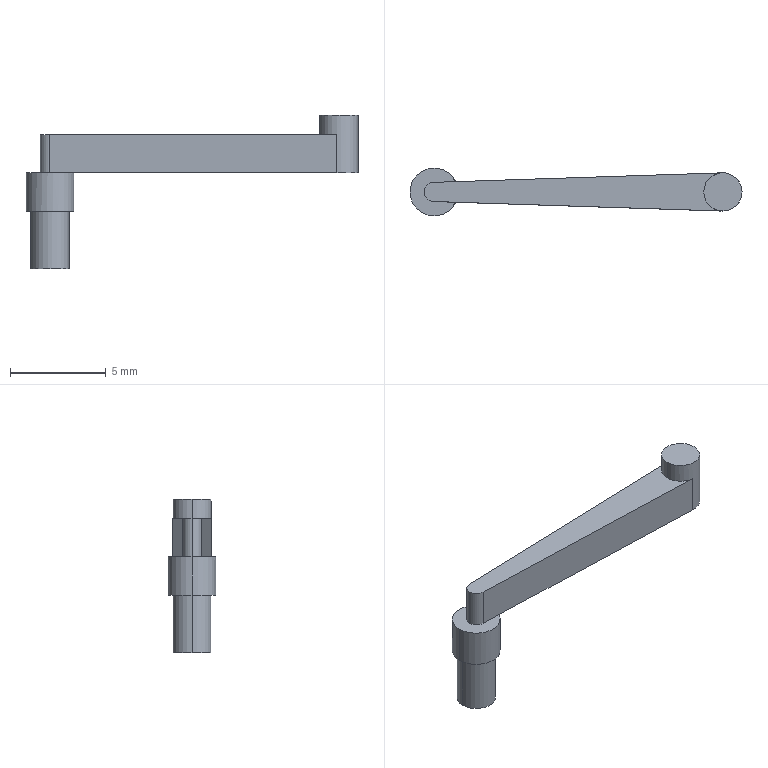Part | SolidWorks | features ICE 5, Extrusion 1 | 1 solid | 16 faces | box 17.35 x 2.5 x 8 mm | volume 71.56 mm3 | cylinder 8 | plane 8 | commonest cylinder face diameters 2 x4 1 x2 2.5 x2
STEP:
#1=CARTESIAN_POINT('',(-1.,0.,-4.));
#2=VERTEX_POINT('',#1);
#3=CARTESIAN_POINT('',(1.,0.,-4.));
#4=VERTEX_POINT('',#3);
#5=CARTESIAN_POINT('',(0.,0.,-4.));
#6=DIRECTION('',(0.,0.,-1.));
#7=DIRECTION('',(-1.,0.,0.));
#8=AXIS2_PLACEMENT_3D('',#5,#6,#7);
#9=CIRCLE('',#8,1.);
#10=EDGE_CURVE('',#2,#4,#9,.T.);
#11=ORIENTED_EDGE('',*,*,#10,.F.);
#12=CARTESIAN_POINT('',(-1.,0.,-1.));
#13=VERTEX_POINT('',#12);
#14=CARTESIAN_POINT('',(-1.,0.,-4.));
#15=DIRECTION('',(0.,0.,1.));
#16=VECTOR('',#15,1000.);
#17=LINE('',#14,#16);
#18=EDGE_CURVE('',#2,#13,#17,.T.);
#19=ORIENTED_EDGE('',*,*,#18,.T.);
#20=CARTESIAN_POINT('',(1.,0.,-1.));
#21=VERTEX_POINT('',#20);
#22=CARTESIAN_POINT('',(0.,0.,-1.));
#23=DIRECTION('',(0.,0.,-1.));
#24=DIRECTION('',(-1.,0.,0.));
#25=AXIS2_PLACEMENT_3D('',#22,#23,#24);
#26=CIRCLE('',#25,1.);
#27=EDGE_CURVE('',#13,#21,#26,.T.);
#28=ORIENTED_EDGE('',*,*,#27,.T.);
#29=CARTESIAN_POINT('',(1.,0.,-4.));
#30=DIRECTION('',(0.,0.,1.));
#31=VECTOR('',#30,1000.);
#32=LINE('',#29,#31);
#33=EDGE_CURVE('',#4,#21,#32,.T.);
#34=ORIENTED_EDGE('',*,*,#33,.F.);
#35=EDGE_LOOP('',(#11,#19,#28,#34));
#36=FACE_OUTER_BOUND('',#35,.T.);
#37=CARTESIAN_POINT('',(0.,0.,-4.));
#38=DIRECTION('',(0.,0.,1.));
#39=DIRECTION('',(1.,0.,0.));
#40=AXIS2_PLACEMENT_3D('',#37,#38,#39);
#41=CYLINDRICAL_SURFACE('',#40,1.);
#42=ADVANCED_FACE('',(#36),#41,.T.);
#43=CARTESIAN_POINT('',(1.25,0.,-1.));
#44=VERTEX_POINT('',#43);
#45=CARTESIAN_POINT('',(-1.25,0.,-1.));
#46=VERTEX_POINT('',#45);
#47=CARTESIAN_POINT('',(0.,0.,-1.));
#48=DIRECTION('',(0.,0.,1.));
#49=DIRECTION('',(1.,0.,0.));
#50=AXIS2_PLACEMENT_3D('',#47,#48,#49);
#51=CIRCLE('',#50,1.25);
#52=EDGE_CURVE('',#44,#46,#51,.T.);
#53=ORIENTED_EDGE('',*,*,#52,.T.);
#54=CARTESIAN_POINT('',(-1.25,0.,1.));
#55=VERTEX_POINT('',#54);
#56=CARTESIAN_POINT('',(-1.25,0.,-1.));
#57=DIRECTION('',(0.,0.,1.));
#58=VECTOR('',#57,1000.);
#59=LINE('',#56,#58);
#60=EDGE_CURVE('',#46,#55,#59,.T.);
#61=ORIENTED_EDGE('',*,*,#60,.T.);
#62=CARTESIAN_POINT('',(1.129,0.5372,1.));
#63=VERTEX_POINT('',#62);
#64=CARTESIAN_POINT('',(0.,0.,1.));
#65=DIRECTION('',(0.,0.,1.));
#66=DIRECTION('',(1.,0.,0.));
#67=AXIS2_PLACEMENT_3D('',#64,#65,#66);
#68=CIRCLE('',#67,1.25);
#69=EDGE_CURVE('',#63,#55,#68,.T.);
#70=ORIENTED_EDGE('',*,*,#69,.F.);
#71=CARTESIAN_POINT('',(1.25,0.,1.));
#72=VERTEX_POINT('',#71);
#73=CARTESIAN_POINT('',(0.,0.,1.));
#74=DIRECTION('',(0.,0.,1.));
#75=DIRECTION('',(1.,0.,0.));
#76=AXIS2_PLACEMENT_3D('',#73,#74,#75);
#77=CIRCLE('',#76,1.25);
#78=EDGE_CURVE('',#72,#63,#77,.T.);
#79=ORIENTED_EDGE('',*,*,#78,.F.);
#80=CARTESIAN_POINT('',(1.25,0.,-1.));
#81=DIRECTION('',(0.,0.,1.));
#82=VECTOR('',#81,1000.);
#83=LINE('',#80,#82);
#84=EDGE_CURVE('',#44,#72,#83,.T.);
#85=ORIENTED_EDGE('',*,*,#84,.F.);
#86=EDGE_LOOP('',(#53,#61,#70,#79,#85));
#87=FACE_OUTER_BOUND('',#86,.T.);
#88=CARTESIAN_POINT('',(0.,0.,-1.));
#89=DIRECTION('',(0.,0.,1.));
#90=DIRECTION('',(1.,0.,0.));
#91=AXIS2_PLACEMENT_3D('',#88,#89,#90);
#92=CYLINDRICAL_SURFACE('',#91,1.25);
#93=ADVANCED_FACE('',(#87),#92,.T.);
#94=CARTESIAN_POINT('',(16.1,0.,4.));
#95=VERTEX_POINT('',#94);
#96=CARTESIAN_POINT('',(14.1,0.,4.));
#97=VERTEX_POINT('',#96);
#98=CARTESIAN_POINT('',(15.1,0.,4.));
#99=DIRECTION('',(0.,0.,1.));
#100=DIRECTION('',(1.,0.,0.));
#101=AXIS2_PLACEMENT_3D('',#98,#99,#100);
#102=CIRCLE('',#101,1.);
#103=EDGE_CURVE('',#95,#97,#102,.T.);
#104=ORIENTED_EDGE('',*,*,#103,.F.);
#105=CARTESIAN_POINT('',(16.1,0.,1.));
#106=VERTEX_POINT('',#105);
#107=CARTESIAN_POINT('',(16.1,0.,3.));
#108=DIRECTION('',(0.,0.,-1.));
#109=VECTOR('',#108,1000.);
#110=LINE('',#107,#109);
#111=EDGE_CURVE('',#95,#106,#110,.T.);
#112=ORIENTED_EDGE('',*,*,#111,.T.);
#113=CARTESIAN_POINT('',(15.,0.995,1.));
#114=VERTEX_POINT('',#113);
#115=CARTESIAN_POINT('',(15.1,0.,1.));
#116=DIRECTION('',(0.,0.,1.));
#117=DIRECTION('',(1.,0.,0.));
#118=AXIS2_PLACEMENT_3D('',#115,#116,#117);
#119=CIRCLE('',#118,1.);
#120=EDGE_CURVE('',#106,#114,#119,.T.);
#121=ORIENTED_EDGE('',*,*,#120,.T.);
#122=CARTESIAN_POINT('',(15.,0.995,3.));
#123=VERTEX_POINT('',#122);
#124=CARTESIAN_POINT('',(15.,0.995,3.));
#125=DIRECTION('',(0.,0.,-1.));
#126=VECTOR('',#125,1000.);
#127=LINE('',#124,#126);
#128=EDGE_CURVE('',#123,#114,#127,.T.);
#129=ORIENTED_EDGE('',*,*,#128,.F.);
#130=CARTESIAN_POINT('',(14.1,0.,3.));
#131=VERTEX_POINT('',#130);
#132=CARTESIAN_POINT('',(15.1,0.,3.));
#133=DIRECTION('',(0.,0.,1.));
#134=DIRECTION('',(1.,0.,0.));
#135=AXIS2_PLACEMENT_3D('',#132,#133,#134);
#136=CIRCLE('',#135,1.);
#137=EDGE_CURVE('',#123,#131,#136,.T.);
#138=ORIENTED_EDGE('',*,*,#137,.T.);
#139=CARTESIAN_POINT('',(14.1,0.,3.));
#140=DIRECTION('',(0.,0.,-1.));
#141=VECTOR('',#140,1000.);
#142=LINE('',#139,#141);
#143=EDGE_CURVE('',#97,#131,#142,.T.);
#144=ORIENTED_EDGE('',*,*,#143,.F.);
#145=EDGE_LOOP('',(#104,#112,#121,#129,#138,#144));
#146=FACE_OUTER_BOUND('',#145,.T.);
#147=CARTESIAN_POINT('',(15.1,0.,3.));
#148=DIRECTION('',(0.,0.,-1.));
#149=DIRECTION('',(-1.,0.,0.));
#150=AXIS2_PLACEMENT_3D('',#147,#148,#149);
#151=CYLINDRICAL_SURFACE('',#150,1.);
#152=ADVANCED_FACE('',(#146),#151,.T.);
#153=CARTESIAN_POINT('',(-0.5,0.,3.));
#154=VERTEX_POINT('',#153);
#155=CARTESIAN_POINT('',(0.,-0.5,3.));
#156=VERTEX_POINT('',#155);
#157=CARTESIAN_POINT('',(0.,0.,3.));
#158=DIRECTION('',(0.,0.,1.));
#159=DIRECTION('',(1.,0.,0.));
#160=AXIS2_PLACEMENT_3D('',#157,#158,#159);
#161=CIRCLE('',#160,0.5);
#162=EDGE_CURVE('',#154,#156,#161,.T.);
#163=ORIENTED_EDGE('',*,*,#162,.F.);
#164=CARTESIAN_POINT('',(-0.5,0.,1.));
#165=VERTEX_POINT('',#164);
#166=CARTESIAN_POINT('',(-0.5,0.,3.));
#167=DIRECTION('',(0.,0.,-1.));
#168=VECTOR('',#167,1000.);
#169=LINE('',#166,#168);
#170=EDGE_CURVE('',#154,#165,#169,.T.);
#171=ORIENTED_EDGE('',*,*,#170,.T.);
#172=CARTESIAN_POINT('',(0.,-0.5,1.));
#173=VERTEX_POINT('',#172);
#174=CARTESIAN_POINT('',(0.,0.,1.));
#175=DIRECTION('',(0.,0.,1.));
#176=DIRECTION('',(1.,0.,0.));
#177=AXIS2_PLACEMENT_3D('',#174,#175,#176);
#178=CIRCLE('',#177,0.5);
#179=EDGE_CURVE('',#165,#173,#178,.T.);
#180=ORIENTED_EDGE('',*,*,#179,.T.);
#181=CARTESIAN_POINT('',(0.,-0.5,3.));
#182=DIRECTION('',(0.,0.,-1.));
#183=VECTOR('',#182,1000.);
#184=LINE('',#181,#183);
#185=EDGE_CURVE('',#156,#173,#184,.T.);
#186=ORIENTED_EDGE('',*,*,#185,.F.);
#187=EDGE_LOOP('',(#163,#171,#180,#186));
#188=FACE_OUTER_BOUND('',#187,.T.);
#189=CARTESIAN_POINT('',(0.,0.,3.));
#190=DIRECTION('',(0.,0.,-1.));
#191=DIRECTION('',(-1.,0.,0.));
#192=AXIS2_PLACEMENT_3D('',#189,#190,#191);
#193=CYLINDRICAL_SURFACE('',#192,0.5);
#194=ADVANCED_FACE('',(#188),#193,.T.);
#195=CARTESIAN_POINT('',(0.,0.5,1.));
#196=VERTEX_POINT('',#195);
#197=CARTESIAN_POINT('',(0.,0.5,1.));
#198=DIRECTION('',(-0.9995,-0.03298,0.));
#199=VECTOR('',#198,1000.);
#200=LINE('',#197,#199);
#201=EDGE_CURVE('',#63,#196,#200,.T.);
#202=ORIENTED_EDGE('',*,*,#201,.F.);
#203=ORIENTED_EDGE('',*,*,#69,.T.);
#204=CARTESIAN_POINT('',(1.129,-0.5372,1.));
#205=VERTEX_POINT('',#204);
#206=CARTESIAN_POINT('',(0.,0.,1.));
#207=DIRECTION('',(0.,0.,1.));
#208=DIRECTION('',(1.,0.,0.));
#209=AXIS2_PLACEMENT_3D('',#206,#207,#208);
#210=CIRCLE('',#209,1.25);
#211=EDGE_CURVE('',#55,#205,#210,.T.);
#212=ORIENTED_EDGE('',*,*,#211,.T.);
#213=CARTESIAN_POINT('',(0.,-0.5,1.));
#214=DIRECTION('',(0.9995,-0.03298,0.));
#215=VECTOR('',#214,1000.);
#216=LINE('',#213,#215);
#217=EDGE_CURVE('',#173,#205,#216,.T.);
#218=ORIENTED_EDGE('',*,*,#217,.F.);
#219=ORIENTED_EDGE('',*,*,#179,.F.);
#220=CARTESIAN_POINT('',(0.,0.,1.));
#221=DIRECTION('',(0.,0.,1.));
#222=DIRECTION('',(1.,0.,0.));
#223=AXIS2_PLACEMENT_3D('',#220,#221,#222);
#224=CIRCLE('',#223,0.5);
#225=EDGE_CURVE('',#196,#165,#224,.T.);
#226=ORIENTED_EDGE('',*,*,#225,.F.);
#227=EDGE_LOOP('',(#202,#203,#212,#218,#219,#226));
#228=FACE_OUTER_BOUND('',#227,.T.);
#229=CARTESIAN_POINT('',(0.,0.,1.));
#230=DIRECTION('',(0.,0.,1.));
#231=DIRECTION('',(1.,0.,0.));
#232=AXIS2_PLACEMENT_3D('',#229,#230,#231);
#233=PLANE('',#232);
#234=ADVANCED_FACE('',(#228),#233,.T.);
#235=CARTESIAN_POINT('',(0.,0.,1.));
#236=DIRECTION('',(0.,0.,1.));
#237=DIRECTION('',(1.,0.,0.));
#238=AXIS2_PLACEMENT_3D('',#235,#236,#237);
#239=CIRCLE('',#238,1.25);
#240=EDGE_CURVE('',#205,#72,#239,.T.);
#241=ORIENTED_EDGE('',*,*,#240,.T.);
#242=ORIENTED_EDGE('',*,*,#78,.T.);
#243=CARTESIAN_POINT('',(0.,0.5,1.));
#244=DIRECTION('',(-0.9995,-0.03298,0.));
#245=VECTOR('',#244,1000.);
#246=LINE('',#243,#245);
#247=EDGE_CURVE('',#114,#63,#246,.T.);
#248=ORIENTED_EDGE('',*,*,#247,.F.);
#249=ORIENTED_EDGE('',*,*,#120,.F.);
#250=CARTESIAN_POINT('',(15.,-0.995,1.));
#251=VERTEX_POINT('',#250);
#252=CARTESIAN_POINT('',(15.1,0.,1.));
#253=DIRECTION('',(0.,0.,1.));
#254=DIRECTION('',(1.,0.,0.));
#255=AXIS2_PLACEMENT_3D('',#252,#253,#254);
#256=CIRCLE('',#255,1.);
#257=EDGE_CURVE('',#251,#106,#256,.T.);
#258=ORIENTED_EDGE('',*,*,#257,.F.);
#259=CARTESIAN_POINT('',(0.,-0.5,1.));
#260=DIRECTION('',(0.9995,-0.03298,0.));
#261=VECTOR('',#260,1000.);
#262=LINE('',#259,#261);
#263=EDGE_CURVE('',#205,#251,#262,.T.);
#264=ORIENTED_EDGE('',*,*,#263,.F.);
#265=EDGE_LOOP('',(#241,#242,#248,#249,#258,#264));
#266=FACE_OUTER_BOUND('',#265,.T.);
#267=CARTESIAN_POINT('',(0.,0.,1.));
#268=DIRECTION('',(0.,0.,1.));
#269=DIRECTION('',(1.,0.,0.));
#270=AXIS2_PLACEMENT_3D('',#267,#268,#269);
#271=PLANE('',#270);
#272=ADVANCED_FACE('',(#266),#271,.F.);
#273=ORIENTED_EDGE('',*,*,#170,.F.);
#274=CARTESIAN_POINT('',(0.,0.5,3.));
#275=VERTEX_POINT('',#274);
#276=CARTESIAN_POINT('',(0.,0.,3.));
#277=DIRECTION('',(0.,0.,1.));
#278=DIRECTION('',(1.,0.,0.));
#279=AXIS2_PLACEMENT_3D('',#276,#277,#278);
#280=CIRCLE('',#279,0.5);
#281=EDGE_CURVE('',#275,#154,#280,.T.);
#282=ORIENTED_EDGE('',*,*,#281,.F.);
#283=CARTESIAN_POINT('',(0.,0.5,3.));
#284=DIRECTION('',(0.,0.,-1.));
#285=VECTOR('',#284,1000.);
#286=LINE('',#283,#285);
#287=EDGE_CURVE('',#275,#196,#286,.T.);
#288=ORIENTED_EDGE('',*,*,#287,.T.);
#289=ORIENTED_EDGE('',*,*,#225,.T.);
#290=EDGE_LOOP('',(#273,#282,#288,#289));
#291=FACE_OUTER_BOUND('',#290,.T.);
#292=CARTESIAN_POINT('',(0.,0.,3.));
#293=DIRECTION('',(0.,0.,-1.));
#294=DIRECTION('',(-1.,0.,0.));
#295=AXIS2_PLACEMENT_3D('',#292,#293,#294);
#296=CYLINDRICAL_SURFACE('',#295,0.5);
#297=ADVANCED_FACE('',(#291),#296,.T.);
#298=ORIENTED_EDGE('',*,*,#217,.T.);
#299=ORIENTED_EDGE('',*,*,#263,.T.);
#300=CARTESIAN_POINT('',(15.,-0.995,3.));
#301=VERTEX_POINT('',#300);
#302=CARTESIAN_POINT('',(15.,-0.995,3.));
#303=DIRECTION('',(0.,0.,-1.));
#304=VECTOR('',#303,1000.);
#305=LINE('',#302,#304);
#306=EDGE_CURVE('',#301,#251,#305,.T.);
#307=ORIENTED_EDGE('',*,*,#306,.F.);
#308=CARTESIAN_POINT('',(0.,-0.5,3.));
#309=DIRECTION('',(0.9995,-0.03298,0.));
#310=VECTOR('',#309,1000.);
#311=LINE('',#308,#310);
#312=EDGE_CURVE('',#156,#301,#311,.T.);
#313=ORIENTED_EDGE('',*,*,#312,.F.);
#314=ORIENTED_EDGE('',*,*,#185,.T.);
#315=EDGE_LOOP('',(#298,#299,#307,#313,#314));
#316=FACE_OUTER_BOUND('',#315,.T.);
#317=CARTESIAN_POINT('',(0.,-0.5,3.));
#318=DIRECTION('',(0.03298,0.9995,0.));
#319=DIRECTION('',(-0.9995,0.03298,0.));
#320=AXIS2_PLACEMENT_3D('',#317,#318,#319);
#321=PLANE('',#320);
#322=ADVANCED_FACE('',(#316),#321,.F.);
#323=ORIENTED_EDGE('',*,*,#111,.F.);
#324=CARTESIAN_POINT('',(15.1,0.,4.));
#325=DIRECTION('',(0.,0.,1.));
#326=DIRECTION('',(1.,0.,0.));
#327=AXIS2_PLACEMENT_3D('',#324,#325,#326);
#328=CIRCLE('',#327,1.);
#329=EDGE_CURVE('',#97,#95,#328,.T.);
#330=ORIENTED_EDGE('',*,*,#329,.F.);
#331=ORIENTED_EDGE('',*,*,#143,.T.);
#332=CARTESIAN_POINT('',(15.1,0.,3.));
#333=DIRECTION('',(0.,0.,1.));
#334=DIRECTION('',(1.,0.,0.));
#335=AXIS2_PLACEMENT_3D('',#332,#333,#334);
#336=CIRCLE('',#335,1.);
#337=EDGE_CURVE('',#131,#301,#336,.T.);
#338=ORIENTED_EDGE('',*,*,#337,.T.);
#339=ORIENTED_EDGE('',*,*,#306,.T.);
#340=ORIENTED_EDGE('',*,*,#257,.T.);
#341=EDGE_LOOP('',(#323,#330,#331,#338,#339,#340));
#342=FACE_OUTER_BOUND('',#341,.T.);
#343=CARTESIAN_POINT('',(15.1,0.,3.));
#344=DIRECTION('',(0.,0.,-1.));
#345=DIRECTION('',(-1.,0.,0.));
#346=AXIS2_PLACEMENT_3D('',#343,#344,#345);
#347=CYLINDRICAL_SURFACE('',#346,1.);
#348=ADVANCED_FACE('',(#342),#347,.T.);
#349=ORIENTED_EDGE('',*,*,#247,.T.);
#350=ORIENTED_EDGE('',*,*,#201,.T.);
#351=ORIENTED_EDGE('',*,*,#287,.F.);
#352=CARTESIAN_POINT('',(0.,0.5,3.));
#353=DIRECTION('',(-0.9995,-0.03298,0.));
#354=VECTOR('',#353,1000.);
#355=LINE('',#352,#354);
#356=EDGE_CURVE('',#123,#275,#355,.T.);
#357=ORIENTED_EDGE('',*,*,#356,.F.);
#358=ORIENTED_EDGE('',*,*,#128,.T.);
#359=EDGE_LOOP('',(#349,#350,#351,#357,#358));
#360=FACE_OUTER_BOUND('',#359,.T.);
#361=CARTESIAN_POINT('',(0.,0.5,3.));
#362=DIRECTION('',(0.03298,-0.9995,0.));
#363=DIRECTION('',(0.9995,0.03298,0.));
#364=AXIS2_PLACEMENT_3D('',#361,#362,#363);
#365=PLANE('',#364);
#366=ADVANCED_FACE('',(#360),#365,.F.);
#367=ORIENTED_EDGE('',*,*,#137,.F.);
#368=ORIENTED_EDGE('',*,*,#356,.T.);
#369=ORIENTED_EDGE('',*,*,#281,.T.);
#370=ORIENTED_EDGE('',*,*,#162,.T.);
#371=ORIENTED_EDGE('',*,*,#312,.T.);
#372=ORIENTED_EDGE('',*,*,#337,.F.);
#373=EDGE_LOOP('',(#367,#368,#369,#370,#371,#372));
#374=FACE_OUTER_BOUND('',#373,.T.);
#375=CARTESIAN_POINT('',(0.,0.,3.));
#376=DIRECTION('',(0.,0.,1.));
#377=DIRECTION('',(1.,0.,0.));
#378=AXIS2_PLACEMENT_3D('',#375,#376,#377);
#379=PLANE('',#378);
#380=ADVANCED_FACE('',(#374),#379,.T.);
#381=ORIENTED_EDGE('',*,*,#329,.T.);
#382=ORIENTED_EDGE('',*,*,#103,.T.);
#383=EDGE_LOOP('',(#381,#382));
#384=FACE_OUTER_BOUND('',#383,.T.);
#385=CARTESIAN_POINT('',(15.1,0.,4.));
#386=DIRECTION('',(0.,0.,1.));
#387=DIRECTION('',(1.,0.,0.));
#388=AXIS2_PLACEMENT_3D('',#385,#386,#387);
#389=PLANE('',#388);
#390=ADVANCED_FACE('',(#384),#389,.T.);
#391=CARTESIAN_POINT('',(0.,0.,-1.));
#392=DIRECTION('',(0.,0.,-1.));
#393=DIRECTION('',(-1.,0.,0.));
#394=AXIS2_PLACEMENT_3D('',#391,#392,#393);
#395=CIRCLE('',#394,1.);
#396=EDGE_CURVE('',#21,#13,#395,.T.);
#397=ORIENTED_EDGE('',*,*,#396,.F.);
#398=ORIENTED_EDGE('',*,*,#27,.F.);
#399=EDGE_LOOP('',(#397,#398));
#400=FACE_BOUND('',#399,.T.);
#401=ORIENTED_EDGE('',*,*,#52,.F.);
#402=CARTESIAN_POINT('',(0.,0.,-1.));
#403=DIRECTION('',(0.,0.,1.));
#404=DIRECTION('',(1.,0.,0.));
#405=AXIS2_PLACEMENT_3D('',#402,#403,#404);
#406=CIRCLE('',#405,1.25);
#407=EDGE_CURVE('',#46,#44,#406,.T.);
#408=ORIENTED_EDGE('',*,*,#407,.F.);
#409=EDGE_LOOP('',(#401,#408));
#410=FACE_OUTER_BOUND('',#409,.T.);
#411=CARTESIAN_POINT('',(0.,0.,-1.));
#412=DIRECTION('',(0.,0.,1.));
#413=DIRECTION('',(1.,0.,0.));
#414=AXIS2_PLACEMENT_3D('',#411,#412,#413);
#415=PLANE('',#414);
#416=ADVANCED_FACE('',(#400,#410),#415,.F.);
#417=ORIENTED_EDGE('',*,*,#60,.F.);
#418=ORIENTED_EDGE('',*,*,#407,.T.);
#419=ORIENTED_EDGE('',*,*,#84,.T.);
#420=ORIENTED_EDGE('',*,*,#240,.F.);
#421=ORIENTED_EDGE('',*,*,#211,.F.);
#422=EDGE_LOOP('',(#417,#418,#419,#420,#421));
#423=FACE_OUTER_BOUND('',#422,.T.);
#424=CARTESIAN_POINT('',(0.,0.,-1.));
#425=DIRECTION('',(0.,0.,1.));
#426=DIRECTION('',(1.,0.,0.));
#427=AXIS2_PLACEMENT_3D('',#424,#425,#426);
#428=CYLINDRICAL_SURFACE('',#427,1.25);
#429=ADVANCED_FACE('',(#423),#428,.T.);
#430=ORIENTED_EDGE('',*,*,#18,.F.);
#431=CARTESIAN_POINT('',(0.,0.,-4.));
#432=DIRECTION('',(0.,0.,-1.));
#433=DIRECTION('',(-1.,0.,0.));
#434=AXIS2_PLACEMENT_3D('',#431,#432,#433);
#435=CIRCLE('',#434,1.);
#436=EDGE_CURVE('',#4,#2,#435,.T.);
#437=ORIENTED_EDGE('',*,*,#436,.F.);
#438=ORIENTED_EDGE('',*,*,#33,.T.);
#439=ORIENTED_EDGE('',*,*,#396,.T.);
#440=EDGE_LOOP('',(#430,#437,#438,#439));
#441=FACE_OUTER_BOUND('',#440,.T.);
#442=CARTESIAN_POINT('',(0.,0.,-4.));
#443=DIRECTION('',(0.,0.,1.));
#444=DIRECTION('',(1.,0.,0.));
#445=AXIS2_PLACEMENT_3D('',#442,#443,#444);
#446=CYLINDRICAL_SURFACE('',#445,1.);
#447=ADVANCED_FACE('',(#441),#446,.T.);
#448=ORIENTED_EDGE('',*,*,#436,.T.);
#449=ORIENTED_EDGE('',*,*,#10,.T.);
#450=EDGE_LOOP('',(#448,#449));
#451=FACE_OUTER_BOUND('',#450,.T.);
#452=CARTESIAN_POINT('',(0.,0.,-4.));
#453=DIRECTION('',(0.,0.,-1.));
#454=DIRECTION('',(-1.,0.,0.));
#455=AXIS2_PLACEMENT_3D('',#452,#453,#454);
#456=PLANE('',#455);
#457=ADVANCED_FACE('',(#451),#456,.T.);
#458=CLOSED_SHELL('',(#42,#93,#152,#194,#234,#272,#297,#322,#348,#366,#380,#390,#416,#429,#447,#457));
#459=MANIFOLD_SOLID_BREP('',#458);
#460=CARTESIAN_POINT('',(0.,0.,0.));
#461=DIRECTION('',(0.,0.,1.));
#462=DIRECTION('',(1.,0.,0.));
#463=AXIS2_PLACEMENT_3D('',#460,#461,#462);
#464=(LENGTH_UNIT()NAMED_UNIT(*)SI_UNIT(.MILLI.,.METRE.));
#465=UNCERTAINTY_MEASURE_WITH_UNIT(LENGTH_MEASURE(0.00001),#464,'','');
#466=(NAMED_UNIT(*)PLANE_ANGLE_UNIT()SI_UNIT($,.RADIAN.));
#467=(NAMED_UNIT(*)SI_UNIT($,.STERADIAN.)SOLID_ANGLE_UNIT());
#468=(GEOMETRIC_REPRESENTATION_CONTEXT(3)GLOBAL_UNCERTAINTY_ASSIGNED_CONTEXT((#465))GLOBAL_UNIT_ASSIGNED_CONTEXT((#464,#466,#467))REPRESENTATION_CONTEXT('',''));
#469=ADVANCED_BREP_SHAPE_REPRESENTATION('',(#459,#463),#468);